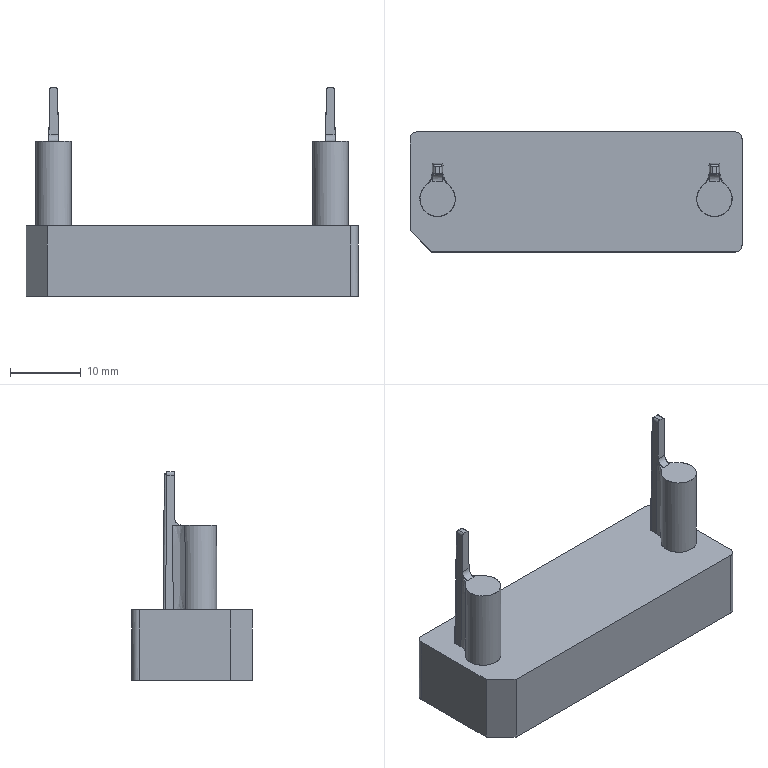NC program | PowerMill | posted with a generic post | part box 47 x 17 x 29.578 mm
Lines 10830 to 11841 of 182382:
N10927 M6
N10928 S18000 M03
N10929 G00 G90 X0.0 Y0.0
N10930 G43 Z10.798 H14
N10931
N10932 G05 P10000 R8
N10933 X20.8197 Y0.1356
N10934 Z0.788
N10935 G01 Z-0.412 F1200.0
N10936 X20.8115 Y0.2066 F2000.0
N10937 X20.7955 Y0.2762
N10938 X20.7717 Y0.3436
N10939 X20.7406 Y0.408
N10940 X20.7026 Y0.4684
N10941 X20.658 Y0.5243
N10942 X20.6075 Y0.5748
N10943 X20.5517 Y0.6194
N10944 X20.4913 Y0.6574
N10945 X20.427 Y0.6885
N10946 X20.3595 Y0.7123
N10947 X20.2899 Y0.7284
N10948 X20.219 Y0.7366
N10949 X20.1475 Y0.7369
N10950 X20.143 Y0.7366
N10951 X20.0067 Y0.7286
N10952 X19.8415 Y0.7259
N10953 X19.6691
N10954 X19.6176 Y0.7257
N10955 X19.5661 Y0.7256
N10956 X19.5084 Y0.7255
N10957 X19.4321 Y0.7254
N10958 X19.3156 Y0.7259
N10959 X19.2319 Y0.7268
N10960 X19.1698 Y0.728
N10961 X19.1184 Y0.7296
N10962 X19.0671 Y0.7324
N10963 X19.0159 Y0.7381
N10964 X18.896 Y0.7576
N10965 X18.7779 Y0.7849
N10966 X18.6623 Y0.8197
N10967 X18.5497 Y0.862
N10968 X18.4406 Y0.9114
N10969 X18.3356 Y0.9677
N10970 X18.2348 Y1.0308
N10971 X18.1384 Y1.1004
N10972 X18.0465 Y1.1765
N10973 X17.9599 Y1.2586
N10974 X17.879 Y1.3462
N10975 X17.804 Y1.4391
N10976 X17.7353 Y1.537
N10977 X17.6731 Y1.6394
N10978 X17.6178 Y1.7458
N10979 X17.5697 Y1.8557
N10980 X17.5291 Y1.9685
N10981 X17.496 Y2.0837
N10982 X17.4707 Y2.2007
N10983 X17.4532 Y2.3191
N10984 X17.4435 Y2.4384
N10985 X17.4415 Y2.5583
N10986 X17.4427 Y3.1516
N10987 X17.4401 Y3.5094
N10988 X17.4424 Y3.6367
N10989 X17.4523 Y3.761
N10990 X17.4697 Y3.8818
N10991 X17.4944 Y3.9989
N10992 X17.5262 Y4.112
N10993 X17.5653 Y4.222
N10994 X17.6127 Y4.3319
N10995 X17.6674 Y4.4383
N10996 X17.729 Y4.541
N10997 X17.7974 Y4.6394
N10998 X17.8722 Y4.7331
N10999 X17.953 Y4.8215
N11000 X18.0394 Y4.9042
N11001 X18.1311 Y4.981
N11002 X18.2277 Y5.0515
N11003 X18.3289 Y5.1153
N11004 X18.4326 Y5.1716
N11005 X18.5402 Y5.2209
N11006 X18.6524 Y5.2636
N11007 X18.769 Y5.2996
N11008 X18.8898 Y5.3285
N11009 X19.0145 Y5.3502
N11010 X19.1427 Y5.3645
N11011 X19.274 Y5.3712
N11012 X19.4079 Y5.371
N11013 X19.8323 Y5.3716
N11014 X19.9716 Y5.3692
N11015 X20.1044 Y5.3594
N11016 X20.231 Y5.3425
N11017 X20.352 Y5.3188
N11018 X20.4682 Y5.2882
N11019 X20.582 Y5.25
N11020 X20.6931 Y5.2044
N11021 X20.8009 Y5.1515
N11022 X20.905 Y5.0916
N11023 X21.0049 Y5.0248
N11024 X21.1001 Y4.9516
N11025 X21.1901 Y4.8724
N11026 X21.2746 Y4.7874
N11027 X21.3532 Y4.697
N11028 X21.4256 Y4.6016
N11029 X21.4899 Y4.5043
N11030 X21.5475 Y4.4027
N11031 X21.5987 Y4.2964
N11032 X21.6432 Y4.1858
N11033 X21.6805 Y4.0714
N11034 X21.7106 Y3.9538
N11035 X21.7331 Y3.8336
N11036 X21.7478 Y3.7114
N11037 X21.7546 Y3.5879
N11038 X21.7541 Y3.4641
N11039 X21.7515 Y3.0801
N11040 X21.753 Y2.53
N11041 X21.7492 Y2.4087
N11042 X21.7375 Y2.2882
N11043 X21.7179 Y2.1691
N11044 X21.6906 Y2.052
N11045 X21.6557 Y1.9375
N11046 X21.6134 Y1.826
N11047 X21.564 Y1.718
N11048 X21.5076 Y1.6137
N11049 X21.4442 Y1.5134
N11050 X21.3735 Y1.4163
N11051 X21.2965 Y1.3241
N11052 X21.2136 Y1.2373
N11053 X21.1252 Y1.1564
N11054 X21.0319 Y1.0817
N11055 X20.9339 Y1.0135
N11056 X20.8316 Y0.952
N11057 X20.7257 Y0.8974
N11058 X20.6161 Y0.8497
N11059 X20.5055 Y0.81
N11060 X20.3943 Y0.7784
N11061 X20.2828 Y0.7549
N11062 X20.1715 Y0.7394
N11063 X20.143 Y0.7366
N11064 X20.0723 Y0.726
N11065 X20.0033 Y0.7075
N11066 X19.9368 Y0.6814
N11067 X19.8736 Y0.648
N11068 X19.8145 Y0.6079
N11069 X19.7603 Y0.5614
N11070 X19.7116 Y0.5091
N11071 X19.669 Y0.4518
N11072 X19.6331 Y0.39
N11073 X19.6042 Y0.3246
N11074 X19.5829 Y0.2564
N11075 X19.5692 Y0.1863
N11076 X19.5635 Y0.1151
N11077 X19.5658 Y0.0437
N11078 X19.5662 Y0.0391
N11079 X20.8236 Y0.1368 Z-0.432
N11080 X20.815 Y0.2077
N11081 X20.7985 Y0.2772
N11082 X20.7744 Y0.3445
N11083 X20.7429 Y0.4086
N11084 X20.7044 Y0.4689
N11085 X20.6595 Y0.5244
N11086 X20.6087 Y0.5746
N11087 X20.5526 Y0.6189
N11088 X20.492 Y0.6566
N11089 X20.4275 Y0.6873
N11090 X20.3599 Y0.7106
N11091 X20.2902 Y0.7263
N11092 X20.2192 Y0.734
N11093 X20.1477 Y0.7339
N11094 X20.1432 Y0.7336
N11095 X20.064 Y0.7284
N11096 X19.9056 Y0.725
N11097 X19.6592 Y0.7247
N11098 X19.1794 Y0.7252
N11099 X19.0602 Y0.7296
N11100 X18.9415 Y0.7421
N11101 X18.824 Y0.7624
N11102 X18.708 Y0.7905
N11103 X18.594 Y0.8264
N11104 X18.4825 Y0.8698
N11105 X18.3742 Y0.9206
N11106 X18.2696 Y0.9785
N11107 X18.1691 Y1.0431
N11108 X18.0733 Y1.1141
N11109 X17.9823 Y1.1915
N11110 X17.8967 Y1.2747
N11111 X17.8168 Y1.3634
N11112 X17.743 Y1.4573
N11113 X17.6754 Y1.5561
N11114 X17.6145 Y1.6593
N11115 X17.5605 Y1.7665
N11116 X17.5138 Y1.8769
N11117 X17.4746 Y1.9902
N11118 X17.443 Y2.1057
N11119 X17.4192 Y2.2229
N11120 X17.4032 Y2.3414
N11121 X17.3951 Y2.4606
N11122 X17.3942 Y2.5803
N11123 X17.3946 Y3.1951
N11124 X17.3922 Y3.5094
N11125 X17.3945 Y3.6358
N11126 X17.4047 Y3.7597
N11127 X17.4224 Y3.8809
N11128 X17.4477 Y3.9993
N11129 X17.4804 Y4.1147
N11130 X17.5205 Y4.2268
N11131 X17.5676 Y4.3355
N11132 X17.6219 Y4.4408
N11133 X17.6832 Y4.5425
N11134 X17.7514 Y4.6405
N11135 X17.8259 Y4.7336
N11136 X17.9065 Y4.8216
N11137 X17.993 Y4.9043
N11138 X18.0852 Y4.9813
N11139 X18.1828 Y5.0524
N11140 X18.2855 Y5.1174
N11141 X18.3831 Y5.1708
N11142 X18.4838 Y5.2182
N11143 X18.5973 Y5.2644
N11144 X18.7025 Y5.3006
N11145 X18.8096 Y5.3306
N11146 X18.931 Y5.3567
N11147 X19.0569 Y5.3757
N11148 X19.187 Y5.3873
N11149 X19.3214 Y5.3914
N11150 X19.4598 Y5.3907
N11151 X19.8323 Y5.3917
N11152 X19.9702 Y5.3894
N11153 X20.1026 Y5.3796
N11154 X20.2296 Y5.3626
N11155 X20.3515 Y5.3387
N11156 X20.4683 Y5.3079
N11157 X20.5822 Y5.2703
N11158 X20.6995 Y5.2236
N11159 X20.8121 Y5.1705
N11160 X20.9197 Y5.1111
N11161 X21.0221 Y5.0455
N11162 X21.1191 Y4.974
N11163 X21.2105 Y4.8969
N11164 X21.2961 Y4.8141
N11165 X21.3757 Y4.7261
N11166 X21.4493 Y4.6331
N11167 X21.5165 Y4.5351
N11168 X21.5774 Y4.4325
N11169 X21.6318 Y4.3255
N11170 X21.6781 Y4.2176
N11171 X21.7172 Y4.107
N11172 X21.749 Y3.9934
N11173 X21.7735 Y3.8766
N11174 X21.7906 Y3.7563
N11175 X21.8003 Y3.6323
N11176 X21.8025 Y3.5094
N11177 X21.8001 Y2.9656
N11178 X21.8008 Y2.53
N11179 X21.7971 Y2.4091
N11180 X21.7854 Y2.2888
N11181 X21.7658 Y2.1699
N11182 X21.7385 Y2.0529
N11183 X21.7036 Y1.9384
N11184 X21.6612 Y1.8268
N11185 X21.6116 Y1.7183
N11186 X21.5548 Y1.6134
N11187 X21.4911 Y1.5124
N11188 X21.4206 Y1.4157
N11189 X21.3436 Y1.3236
N11190 X21.2606 Y1.2368
N11191 X21.172 Y1.1557
N11192 X21.0784 Y1.0806
N11193 X20.9801 Y1.0121
N11194 X20.8778 Y0.9505
N11195 X20.772 Y0.8961
N11196 X20.6634 Y0.8492
N11197 X20.5523 Y0.8098
N11198 X20.4393 Y0.7782
N11199 X20.325 Y0.7544
N11200 X20.2092 Y0.7385
N11201 X20.1922 Y0.7368
N11202 X20.1432 Y0.7336
N11203 X20.0723 Y0.7249
N11204 X20.0028 Y0.7085
N11205 X19.9355 Y0.6843
N11206 X19.8713 Y0.6528
N11207 X19.8111 Y0.6144
N11208 X19.7556 Y0.5695
N11209 X19.7054 Y0.5187
N11210 X19.6611 Y0.4626
N11211 X19.6234 Y0.4019
N11212 X19.5927 Y0.3374
N11213 X19.5694 Y0.2698
N11214 X19.5537 Y0.2001
N11215 X19.5459 Y0.1291
N11216 X19.5461 Y0.0577
N11217 X19.5464 Y0.0531
N11218 X20.8243 Y0.1328 Z-0.452
N11219 X20.8156 Y0.2037
N11220 X20.7991 Y0.2732
N11221 X20.7749 Y0.3404
N11222 X20.7434 Y0.4046
N11223 X20.7049 Y0.4647
N11224 X20.66 Y0.5203
N11225 X20.6091 Y0.5704
N11226 X20.553 Y0.6146
N11227 X20.4923 Y0.6523
N11228 X20.4278 Y0.683
N11229 X20.3602 Y0.7063
N11230 X20.2905 Y0.7219
N11231 X20.2194 Y0.7296
N11232 X20.148 Y0.7294
N11233 X20.1435 Y0.7291
N11234 X20.0898 Y0.7256
N11235 X19.9277 Y0.722
N11236 X19.6972 Y0.7228
N11237 X19.4058 Y0.7236
N11238 X19.122 Y0.7274
N11239 X19.0162 Y0.7302
N11240 X18.9495 Y0.7355
N11241 X18.8833 Y0.7451
N11242 X18.8072 Y0.7596
N11243 X18.7124 Y0.782
N11244 X18.5937 Y0.8162
N11245 X18.5028 Y0.8476
N11246 X18.4312 Y0.8766
N11247 X18.3708 Y0.9052
N11248 X18.2607 Y0.9651
N11249 X18.1563 Y1.0307
N11250 X18.0581 Y1.1017
N11251 X17.9663 Y1.1777
N11252 X17.8811 Y1.2584
N11253 X17.8014 Y1.3446
N11254 X17.7261 Y1.4376
N11255 X17.6571 Y1.5357
N11256 X17.5945 Y1.6384
N11257 X17.5397 Y1.7434
N11258 X17.492 Y1.8518
N11259 X17.4516 Y1.9633
N11260 X17.4186 Y2.0779
N11261 X17.3931 Y2.1949
N11262 X17.3754 Y2.314
N11263 X17.3655 Y2.4346
N11264 X17.3634 Y2.5561
N11265 X17.3659 Y3.1187
N11266 X17.3637 Y3.5022
N11267 X17.3653 Y3.6302
N11268 X17.3747 Y3.7551
N11269 X17.3915 Y3.8765
N11270 X17.4157 Y3.9942
N11271 X17.4469 Y4.1078
N11272 X17.4851 Y4.2172
N11273 X17.53 Y4.3223
N11274 X17.5819 Y4.4242
N11275 X17.644 Y4.5292
N11276 X17.7124 Y4.6293
N11277 X17.7869 Y4.7241
N11278 X17.8672 Y4.8136
N11279 X17.9492 Y4.8934
N11280 X18.0389 Y4.9698
N11281 X18.1368 Y5.0428
N11282 X18.2432 Y5.1124
N11283 X18.3517 Y5.1745
N11284 X18.4641 Y5.2299
N11285 X18.5802 Y5.2782
N11286 X18.6997 Y5.3194
N11287 X18.8224 Y5.3531
N11288 X18.9477 Y5.3794
N11289 X19.0753 Y5.3979
N11290 X19.2046 Y5.4087
N11291 X19.3352 Y5.4115
N11292 X19.4662 Y5.4104
N11293 X19.8323 Y5.4116
N11294 X19.9698 Y5.4093
N11295 X20.1025 Y5.3995
N11296 X20.2304 Y5.3823
N11297 X20.3535 Y5.3581
N11298 X20.4719 Y5.3269
N11299 X20.5869 Y5.2887
N11300 X20.7062 Y5.2406
N11301 X20.822 Y5.1854
N11302 X20.9338 Y5.1233
N11303 X21.0412 Y5.0545
N11304 X21.1379 Y4.9839
N11305 X21.2295 Y4.9078
N11306 X21.3158 Y4.8257
N11307 X21.3966 Y4.7379
N11308 X21.4715 Y4.6446
N11309 X21.5401 Y4.5464
N11310 X21.6022 Y4.4437
N11311 X21.6573 Y4.3371
N11312 X21.7043 Y4.2291
N11313 X21.7442 Y4.118
N11314 X21.7768 Y4.0038
N11315 X21.8021 Y3.8862
N11316 X21.82 Y3.7654
N11317 X21.8304 Y3.6411
N11318 X21.8331 Y3.5133
N11319 X21.832 Y3.3826
N11320 X21.8309 Y2.7953
N11321 X21.8316 Y2.53
N11322 X21.8281 Y2.4092
N11323 X21.8167 Y2.2895
N11324 X21.7975 Y2.1713
N11325 X21.7706 Y2.055
N11326 X21.736 Y1.9408
N11327 X21.6939 Y1.8293
N11328 X21.6444 Y1.7208
N11329 X21.5876 Y1.6157
N11330 X21.5238 Y1.5144
N11331 X21.4532 Y1.4172
N11332 X21.3766 Y1.3251
N11333 X21.2943 Y1.2386
N11334 X21.2066 Y1.1581
N11335 X21.1142 Y1.084
N11336 X21.0174 Y1.0166
N11337 X20.9165 Y0.9557
N11338 X20.8076 Y0.8991
N11339 X20.6973 Y0.8505
N11340 X20.5861 Y0.81
N11341 X20.4746 Y0.7777
N11342 X20.3631 Y0.7534
N11343 X20.252 Y0.7372
N11344 X20.2253 Y0.7345
N11345 X20.1435 Y0.7291
N11346 X20.0726 Y0.7204
N11347 X20.0031 Y0.7039
N11348 X19.9358 Y0.6797
N11349 X19.8717 Y0.6482
N11350 X19.8115 Y0.6097
N11351 X19.756 Y0.5648
N11352 X19.7058 Y0.5139
N11353 X19.6616 Y0.4578
N11354 X19.6239 Y0.3971
N11355 X19.5933 Y0.3326
N11356 X19.57 Y0.265
N11357 X19.5543 Y0.1953
N11358 X19.5466 Y0.1242
N11359 X19.5468 Y0.0528
N11360 X19.5471 Y0.0483
N11361 X20.8256 Y0.1344 Z-0.472
N11362 X20.8168 Y0.2053
N11363 X20.8001 Y0.2747
N11364 X20.7757 Y0.3419
N11365 X20.7441 Y0.406
N11366 X20.7055 Y0.4661
N11367 X20.6604 Y0.5215
N11368 X20.6094 Y0.5716
N11369 X20.5532 Y0.6157
N11370 X20.4925 Y0.6532
N11371 X20.4279 Y0.6837
N11372 X20.3602 Y0.7069
N11373 X20.2905 Y0.7224
N11374 X20.2194 Y0.7299
N11375 X20.148 Y0.7296
N11376 X20.1435 Y0.7293
N11377 X20.1052 Y0.7267
N11378 X19.9591 Y0.7244
N11379 X19.6691
N11380 X19.4067 Y0.7223
N11381 X19.1944
N11382 X19.026 Y0.7278
N11383 X18.9146 Y0.7373
N11384 X18.8014 Y0.7549
N11385 X18.6872 Y0.7806
N11386 X18.573 Y0.8145
N11387 X18.4597 Y0.8564
N11388 X18.3487 Y0.906
N11389 X18.2415 Y0.9626
N11390 X18.139 Y1.0256
N11391 X18.0422 Y1.0943
N11392 X17.9517 Y1.1682
N11393 X17.8676 Y1.2469
N11394 X17.7856 Y1.3345
N11395 X17.7096 Y1.4274
N11396 X17.6398 Y1.5251
N11397 X17.5767 Y1.6274
N11398 X17.5206 Y1.7335
N11399 X17.4717 Y1.8429
N11400 X17.4302 Y1.9554
N11401 X17.3963 Y2.0704
N11402 X17.3705 Y2.1859
N11403 X17.3523 Y2.3034
N11404 X17.3418 Y2.4235
N11405 X17.339 Y2.5456
N11406 X17.3414 Y3.0718
N11407 X17.3406 Y3.4507
N11408 X17.3402 Y3.5858
N11409 X17.3463 Y3.7113
N11410 X17.3592 Y3.8288
N11411 X17.3789 Y3.9396
N11412 X17.4057 Y4.0481
N11413 X17.442 Y4.1625
N11414 X17.4858 Y4.2745
N11415 X17.5372 Y4.3838
N11416 X17.5958 Y4.4898
N11417 X17.6615 Y4.592
N11418 X17.7271 Y4.6811
N11419 X17.7984 Y4.7656
N11420 X17.879 Y4.8495
N11421 X17.9687 Y4.9318
N11422 X18.0669 Y5.0115
N11423 X18.1723 Y5.0867
N11424 X18.2824 Y5.1557
N11425 X18.3946 Y5.2167
N11426 X18.5069 Y5.2691
N11427 X18.6186 Y5.3129
N11428 X18.7388 Y5.3514
N11429 X18.862 Y5.3826
N11430 X18.9878 Y5.4062
N11431 X19.1156 Y5.422
N11432 X19.2449 Y5.43
N11433 X19.3751 Y5.4304
N11434 X19.669 Y5.4301
N11435 X19.8323 Y5.4317
N11436 X19.969 Y5.4294
N11437 X20.1019 Y5.4194
N11438 X20.2309 Y5.402
N11439 X20.3558 Y5.3774
N11440 X20.4767 Y5.3456
N11441 X20.5942 Y5.3066
N11442 X20.7048 Y5.2619
N11443 X20.8161 Y5.2085
N11444 X20.9288 Y5.1459
N11445 X21.0396 Y5.0753
N11446 X21.1433 Y5.0001
N11447 X21.2378 Y4.9224
N11448 X21.3243 Y4.8418
N11449 X21.4056 Y4.7551
N11450 X21.4817 Y4.6626
N11451 X21.5518 Y4.5646
N11452 X21.6154 Y4.4619
N11453 X21.6721 Y4.3555
N11454 X21.7213 Y4.246
N11455 X21.7629 Y4.1343
N11456 X21.7958 Y4.0241
N11457 X21.8213 Y3.9118
N11458 X21.8401 Y3.7938
N11459 X21.8518 Y3.67
N11460 X21.8563 Y3.5397
N11461 X21.8557 Y3.4026
N11462 X21.8553 Y2.7063
N11463 X21.8558 Y2.53
N11464 X21.8523 Y2.4096
N11465 X21.8409 Y2.2901
N11466 X21.8217 Y2.1719
N11467 X21.7947 Y2.0554
N11468 X21.7601 Y1.9411
N11469 X21.718 Y1.8294
N11470 X21.6685 Y1.7207
N11471 X21.6118 Y1.6156
N11472 X21.5482 Y1.5146
N11473 X21.4779 Y1.4179
N11474 X21.4013 Y1.3259
N11475 X21.3186 Y1.239
N11476 X21.2306 Y1.158
N11477 X21.1375 Y1.0831
N11478 X21.0398 Y1.0146
N11479 X20.9379 Y0.9528
N11480 X20.8323 Y0.8981
N11481 X20.7235 Y0.8507
N11482 X20.6121 Y0.8109
N11483 X20.4988 Y0.7789
N11484 X20.3841 Y0.7547
N11485 X20.2684 Y0.7384
N11486 X20.251 Y0.7366
N11487 X20.1435 Y0.7293
N11488 X20.0726 Y0.7204
N11489 X20.0031 Y0.7038
N11490 X19.9359 Y0.6794
N11491 X19.8718 Y0.6477
N11492 X19.8117 Y0.6091
N11493 X19.7563 Y0.5641
N11494 X19.7062 Y0.5131
N11495 X19.6622 Y0.4569
N11496 X19.6246 Y0.3961
N11497 X19.5941 Y0.3315
N11498 X19.5709 Y0.2639
N11499 X19.5555 Y0.1941
N11500 X19.5479 Y0.1231
N11501 X19.5483 Y0.0517
N11502 X19.5486 Y0.0471
N11503 X20.7962 Y0.0991 Z-0.492
N11504 X20.7908 Y0.1703
N11505 X20.7775 Y0.2405
N11506 X20.7564 Y0.3087
N11507 X20.7279 Y0.3743
N11508 X20.6922 Y0.4362
N11509 X20.6499 Y0.4937
N11510 X20.6014 Y0.5462
N11511 X20.5473 Y0.5929
N11512 X20.4884 Y0.6334
N11513 X20.4252 Y0.667
N11514 X20.3617 Y0.6923
N11515 X20.2948 Y0.7106
N11516 X20.2235 Y0.722
N11517 X20.1478 Y0.7261
N11518 X20.1435
N11519 X20.0362 Y0.724
N11520 X19.84 Y0.7244
N11521 X19.5248 Y0.7236
N11522 X19.2439 Y0.7224
N11523 X19.0384 Y0.7261
N11524 X18.9406 Y0.7321
N11525 X18.836 Y0.7461
N11526 X18.719 Y0.7692
N11527 X18.6055 Y0.7981
N11528 X18.494 Y0.8347
N11529 X18.3845 Y0.879
N11530 X18.2777 Y0.9308
N11531 X18.174 Y0.99
N11532 X18.074 Y1.0563
N11533 X17.9792 Y1.1286
N11534 X17.8892 Y1.2071
N11535 X17.8047 Y1.2915
N11536 X17.726 Y1.3813
N11537 X17.6534 Y1.4761
N11538 X17.5872 Y1.5758
N11539 X17.5276 Y1.6798
N11540 X17.4751 Y1.7876
N11541 X17.4299 Y1.8987
N11542 X17.3922 Y2.0124
N11543 X17.3622 Y2.1283
N11544 X17.3399 Y2.2458
N11545 X17.3255 Y2.3645
N11546 X17.319 Y2.4838
N11547 X17.3189 Y2.6036
N11548 X17.3196 Y3.3078
N11549 X17.3186 Y3.5094
N11550 X17.3214 Y3.6415
N11551 X17.3313 Y3.766
N11552 X17.3481 Y3.8836
N11553 X17.3717 Y3.9951
N11554 X17.4025 Y4.1049
N11555 X17.4424 Y4.2184
N11556 X17.4897 Y4.3289
N11557 X17.5442 Y4.4358
N11558 X17.6055 Y4.5387
N11559 X17.6736 Y4.6372
N11560 X17.7465 Y4.7291
N11561 X17.8278 Y4.8191
N11562 X17.9182 Y4.9075
N11563 X18.0159 Y4.9919
N11564 X18.1168 Y5.069
N11565 X18.2178 Y5.1367
N11566 X18.3211 Y5.1977
N11567 X18.4313 Y5.2547
N11568 X18.539 Y5.3021
N11569 X18.649 Y5.3433
N11570 X18.7655 Y5.3801
N11571 X18.8745 Y5.4072
N11572 X18.9781 Y5.4255
N11573 X19.0806 Y5.4367
N11574 X19.2417 Y5.4474
N11575 X19.424 Y5.452
N11576 X19.643 Y5.451
N11577 X19.8253 Y5.4499
N11578 X19.9955 Y5.4481
N11579 X20.0644 Y5.4438
N11580 X20.1588 Y5.433
N11581 X20.267 Y5.4174
N11582 X20.3795 Y5.3934
N11583 X20.496 Y5.3606
N11584 X20.615 Y5.3189
N11585 X20.734 Y5.269
N11586 X20.8481 Y5.2126
N11587 X20.9539 Y5.1523
N11588 X21.0457 Y5.0925
N11589 X21.1414 Y5.0219
N11590 X21.2415 Y4.9388
N11591 X21.3346 Y4.8519
N11592 X21.4141 Y4.7688
N11593 X21.4883 Y4.6808
N11594 X21.559 Y4.5847
N11595 X21.6234 Y4.4837
N11596 X21.6812 Y4.3783
N11597 X21.7321 Y4.269
N11598 X21.7762 Y4.1564
N11599 X21.8117 Y4.0448
N11600 X21.8387 Y3.9346
N11601 X21.8575 Y3.8259
N11602 X21.8682 Y3.7189
N11603 X21.872 Y3.6123
N11604 X21.8752 Y3.3426
N11605 X21.8756 Y2.8957
N11606 X21.8762 Y2.53
N11607 X21.8725 Y2.4097
N11608 X21.861 Y2.2899
N11609 X21.8416 Y2.1712
N11610 X21.8143 Y2.0542
N11611 X21.7794 Y1.9393
N11612 X21.737 Y1.8272
N11613 X21.6873 Y1.7185
N11614 X21.6306 Y1.6135
N11615 X21.567 Y1.5125
N11616 X21.4969 Y1.416
N11617 X21.4204 Y1.3243
N11618 X21.3379 Y1.2379
N11619 X21.2498 Y1.157
N11620 X21.1565 Y1.0822
N11621 X21.0583 Y1.0137
N11622 X20.9558 Y0.9519
N11623 X20.8493 Y0.897
N11624 X20.7395 Y0.8494
N11625 X20.6269 Y0.8093
N11626 X20.5119 Y0.7768
N11627 X20.395 Y0.7519
N11628 X20.2767 Y0.7349
N11629 X20.2729 Y0.7345
N11630 X20.1663 Y0.7266
N11631 X20.1435 Y0.7261
N11632 X20.0723 Y0.7207
N11633 X20.0021 Y0.7074
N11634 X19.9338 Y0.6863
N11635 X19.8683 Y0.6578
N11636 X19.8064 Y0.6221
N11637 X19.7489 Y0.5798
N11638 X19.6964 Y0.5313
N11639 X19.6497 Y0.4772
N11640 X19.6092 Y0.4183
N11641 X19.5756 Y0.3552
N11642 X19.5503 Y0.2916
N11643 X19.532 Y0.2248
N11644 X19.5206 Y0.1534
N11645 X19.5165 Y0.0777
N11646 Y0.0734
N11647 X20.8062 Y0.1095 Z-0.512
N11648 X20.7996 Y0.1806
N11649 X20.7852 Y0.2505
N11650 X20.763 Y0.3185
N11651 X20.7334 Y0.3835
N11652 X20.6968 Y0.4449
N11653 X20.6535 Y0.5017
N11654 X20.6042 Y0.5534
N11655 X20.5494 Y0.5992
N11656 X20.4899 Y0.6387
N11657 X20.4263 Y0.6713
N11658 X20.3595 Y0.6966
N11659 X20.2902 Y0.7143
N11660 X20.2195 Y0.7242
N11661 X20.1481 Y0.7261
N11662 X20.1435 Y0.726
N11663 X20.101 Y0.7244
N11664 X20.0056 Y0.7241
N11665 X19.9102
N11666 X19.4268 Y0.7242
N11667 X19.1825 Y0.7241
N11668 X19.016 Y0.7278
N11669 X18.9034 Y0.7345
N11670 X18.8051 Y0.7463
N11671 X18.7029 Y0.7664
N11672 X18.5957 Y0.7953
N11673 X18.4823 Y0.8338
N11674 X18.3636 Y0.8818
N11675 X18.2605 Y0.9311
N11676 X18.1599 Y0.9879
N11677 X18.062 Y1.0523
N11678 X17.9674 Y1.124
N11679 X17.8766 Y1.2029
N11680 X17.792 Y1.2867
N11681 X17.7129 Y1.3763
N11682 X17.6399 Y1.4709
N11683 X17.5734 Y1.5702
N11684 X17.5136 Y1.6738
N11685 X17.4608 Y1.7813
N11686 X17.4152 Y1.8922
N11687 X17.3771 Y2.0058
N11688 X17.3466 Y2.1217
N11689 X17.324 Y2.2392
N11690 X17.3092 Y2.3579
N11691 X17.3023 Y2.4773
N11692 X17.302 Y2.5972
N11693 X17.3016 Y3.183
N11694 X17.3015 Y3.2235
N11695 X17.3014 Y3.2641
N11696 Y3.3154
N11697 X17.3016 Y3.3815
N11698 X17.3023 Y3.471
N11699 X17.3043 Y3.5875
N11700 X17.3067 Y3.6654
N11701 X17.3094 Y3.7248
N11702 X17.3124 Y3.771
N11703 X17.3163 Y3.8112
N11704 X17.3232 Y3.8512
N11705 X17.3543 Y3.9918
N11706 X17.3871 Y4.111
N11707 X17.4231 Y4.2163
N11708 X17.4631 Y4.3114
N11709 X17.5093 Y4.4038
N11710 X17.5709 Y4.5107
N11711 X17.6387 Y4.6125
N11712 X17.7113 Y4.7076
N11713 X17.7897 Y4.798
N11714 X17.8791 Y4.8897
N11715 X17.9766 Y4.9785
N11716 X18.075 Y5.058
N11717 X18.1724 Y5.1274
N11718 X18.2739 Y5.1908
N11719 X18.3875 Y5.2527
N11720 X18.5037 Y5.307
N11721 X18.622 Y5.3537
N11722 X18.742 Y5.3924
N11723 X18.8631 Y5.4233
N11724 X18.9851 Y5.4463
N11725 X19.1083 Y5.4614
N11726 X19.2383 Y5.4696
N11727 X19.3778 Y5.4709
N11728 X19.6691
N11729 X19.8699 Y5.4708
N11730 X20.0193 Y5.4659
N11731 X20.1483 Y5.4555
N11732 X20.2167 Y5.4457
N11733 X20.2846 Y5.4326
N11734 X20.3577 Y5.416
N11735 X20.4639 Y5.3884
N11736 X20.5414 Y5.3653
N11737 X20.6067 Y5.3429
N11738 X20.6706 Y5.3165
N11739 X20.7972 Y5.2574
N11740 X20.9033 Y5.201
N11741 X20.9994 Y5.1423
N11742 X21.1019 Y5.071
N11743 X21.2038 Y4.9907
N11744 X21.302 Y4.9034
N11745 X21.3931 Y4.812
N11746 X21.4756 Y4.7184
N11747 X21.5489 Y4.6241
N11748 X21.6125 Y4.5302
N11749 X21.6694 Y4.4329
N11750 X21.722 Y4.3287
N11751 X21.7705 Y4.2159
N11752 X21.7945 Y4.1529
N11753 X21.8152 Y4.0887
N11754 X21.8332 Y4.0236
N11755 X21.8529 Y3.9406
N11756 X21.8727 Y3.8384
N11757 X21.8833 Y3.7635
N11758 X21.889 Y3.6965
N11759 X21.8901 Y3.6291
N11760 X21.8933 Y3.3585
N11761 X21.8931 Y3.0879
N11762 X21.8933 Y2.53
N11763 X21.8898 Y2.4099
N11764 X21.8783 Y2.2902
N11765 X21.8589 Y2.1716
N11766 X21.8317 Y2.0545
N11767 X21.7968 Y1.9398
N11768 X21.7544 Y1.8278
N11769 X21.7048 Y1.7191
N11770 X21.648 Y1.614
N11771 X21.5844 Y1.5128
N11772 X21.5139 Y1.4159
N11773 X21.4372 Y1.3239
N11774 X21.3545 Y1.2373
N11775 X21.2662 Y1.1563
N11776 X21.1727 Y1.0814
N11777 X21.0744 Y1.0129
N11778 X20.9749 Y0.9529
N11779 X20.8681 Y0.8976
N11780 X20.7585 Y0.8498
N11781 X20.647 Y0.8098
N11782 X20.5341 Y0.7777
N11783 X20.4203 Y0.7535
N11784 X20.3062 Y0.7373
N11785 X20.2914 Y0.7358
N11786 X20.1964 Y0.7279
N11787 X20.1435 Y0.726
N11788 X20.0724 Y0.7194
N11789 X20.0024 Y0.705
N11790 X19.9345 Y0.6828
N11791 X19.8694 Y0.6532
N11792 X19.8081 Y0.6165
N11793 X19.7513 Y0.5733
N11794 X19.6996 Y0.524
N11795 X19.6537 Y0.4692
N11796 X19.6143 Y0.4097
N11797 X19.5817 Y0.3461
N11798 X19.5563 Y0.2792
N11799 X19.5387 Y0.21
N11800 X19.5288 Y0.1393
N11801 X19.5269 Y0.0678
N11802 X19.527 Y0.0633
N11803 X20.7974 Y0.0994 Z-0.532
N11804 X20.7918 Y0.1707
N11805 X20.7784 Y0.2408
N11806 X20.7572 Y0.309
N11807 X20.7285 Y0.3745
N11808 X20.6927 Y0.4364
N11809 X20.6503 Y0.4938
N11810 X20.6017 Y0.5462
N11811 X20.5476 Y0.5928
N11812 X20.4886 Y0.6331
N11813 X20.4255 Y0.6666
N11814 X20.359 Y0.6929
N11815 X20.2901 Y0.7116
N11816 X20.2195 Y0.7224
N11817 X20.1481 Y0.7254
N11818 X20.1435 Y0.7253
N11819 X20.0727 Y0.7237
N11820 X19.8557 Y0.7239
N11821 X19.2822 Y0.7245
N11822 X19.0162 Y0.7268
N11823 X18.9073 Y0.7323
N11824 X18.7971 Y0.7456
N11825 X18.6856 Y0.7671
N11826 X18.5731 Y0.7969
N11827 X18.4601 Y0.8349
N11828 X18.3494 Y0.8803
N11829 X18.2418 Y0.9328
N11830 X18.1379 Y0.9924
N11831 X18.0382 Y1.0587
N11832 X17.9432 Y1.1316
N11833 X17.8532 Y1.2106
N11834 X17.7687 Y1.2955
N11835 X17.69 Y1.3858
N11836 X17.6176 Y1.4811
N11837 X17.5517 Y1.581
N11838 X17.4926 Y1.6851
N11839 X17.4406 Y1.7929
N11840 X17.3959 Y1.9038
N11841 X17.3586 Y2.0178
N11842 X17.329 Y2.1341
N11843 X17.3071 Y2.2522
N11844 X17.2931 Y2.3716
N11845 X17.2871 Y2.4916
N11846 X17.2872 Y2.612
N11847 X17.2899 Y3.1445
N11848 X17.2879 Y3.5094
N11849 X17.2898 Y3.6388
N11850 X17.2993 Y3.7631
N11851 X17.316 Y3.8824
N11852 X17.3397 Y3.9969
N11853 X17.3703 Y4.1065
N11854 X17.408 Y4.2133
N11855 X17.4555 Y4.3242
N11856 X17.5105 Y4.4326
N11857 X17.5729 Y4.5379
N11858 X17.6425 Y4.6399
N11859 X17.7192 Y4.738
N11860 X17.8068 Y4.8369
N11861 X17.8993 Y4.9295
N11862 X17.9966 Y5.0158
N11863 X18.0986 Y5.0956
N11864 X18.2 Y5.1655
N11865 X18.2894 Y5.2205
N11866 X18.3819 Y5.2703
N11867 X18.4527 Y5.3049
N11868 X18.512 Y5.331
N11869 X18.5723 Y5.3548
N11870 X18.6486 Y5.3825
N11871 X18.7311 Y5.4095
N11872 X18.7932 Y5.4273
N11873 X18.8563 Y5.4416
N11874 X18.9233 Y5.4546
N11875 X18.9903 Y5.4674
N11876 X19.0576 Y5.478
N11877 X19.1253 Y5.4846
N11878 X19.1934 Y5.4872
N11879 X19.4816 Y5.4905
N11880 X19.6691 Y5.4908
N11881 X19.8701 Y5.4905
N11882 X20.0141 Y5.486
N11883 X20.1348 Y5.4762
N11884 X20.2469 Y5.46
N11885 X20.3691 Y5.4346
N11886 X20.4902 Y5.4013
N11887 X20.6098 Y5.3601
N11888 X20.7274 Y5.3112
N11889 X20.8425 Y5.2547
N11890 X20.9546 Y5.1908
N11891 X21.0605 Y5.1215
N11892 X21.1622 Y5.0457
N11893 X21.26 Y4.9628
N11894 X21.3536 Y4.8731
N11895 X21.4426 Y4.7768
N11896 X21.5265 Y4.6742
N11897 X21.5976 Y4.5758
N11898 X21.6618 Y4.4733
N11899 X21.719 Y4.367
N11900 X21.7689 Y4.2576
N11901 X21.8114 Y4.1454
N11902 X21.8467 Y4.0316
N11903 X21.8731 Y3.9211
N11904 X21.891 Y3.8137
N11905 X21.9009 Y3.709
N11906 X21.9042 Y3.6049
N11907 X21.9072 Y3.3289
N11908 X21.9076 Y2.8527
N11909 X21.9081 Y2.53
N11910 X21.9045 Y2.4097
N11911 X21.893 Y2.29
N11912 X21.8735 Y2.1713
N11913 X21.8463 Y2.0542
N11914 X21.8114 Y1.9393
N11915 X21.7689 Y1.8271
N11916 X21.7192 Y1.7183
N11917 X21.6625 Y1.6132
N11918 X21.599 Y1.5122
N11919 X21.5288 Y1.4157
N11920 X21.4523 Y1.324
N11921 X21.3697 Y1.2374
N11922 X21.2816 Y1.1566
N11923 X21.1882 Y1.0817
N11924 X21.0901 Y1.0133
N11925 X20.9875 Y0.9515
N11926 X20.881 Y0.8966
N11927 X20.7712 Y0.849
N11928 X20.6585 Y0.8088
N11929 X20.5434 Y0.7763
N11930 X20.4264 Y0.7515
N11931 X20.3081 Y0.7345
N11932 X20.2028 Y0.7266
N11933 X20.1435 Y0.7253
N11934 X20.0723 Y0.7197
N11935 X20.0022 Y0.7063
N11936 X19.9339 Y0.6851
N11937 X19.8684 Y0.6564
N11938 X19.8066 Y0.6206